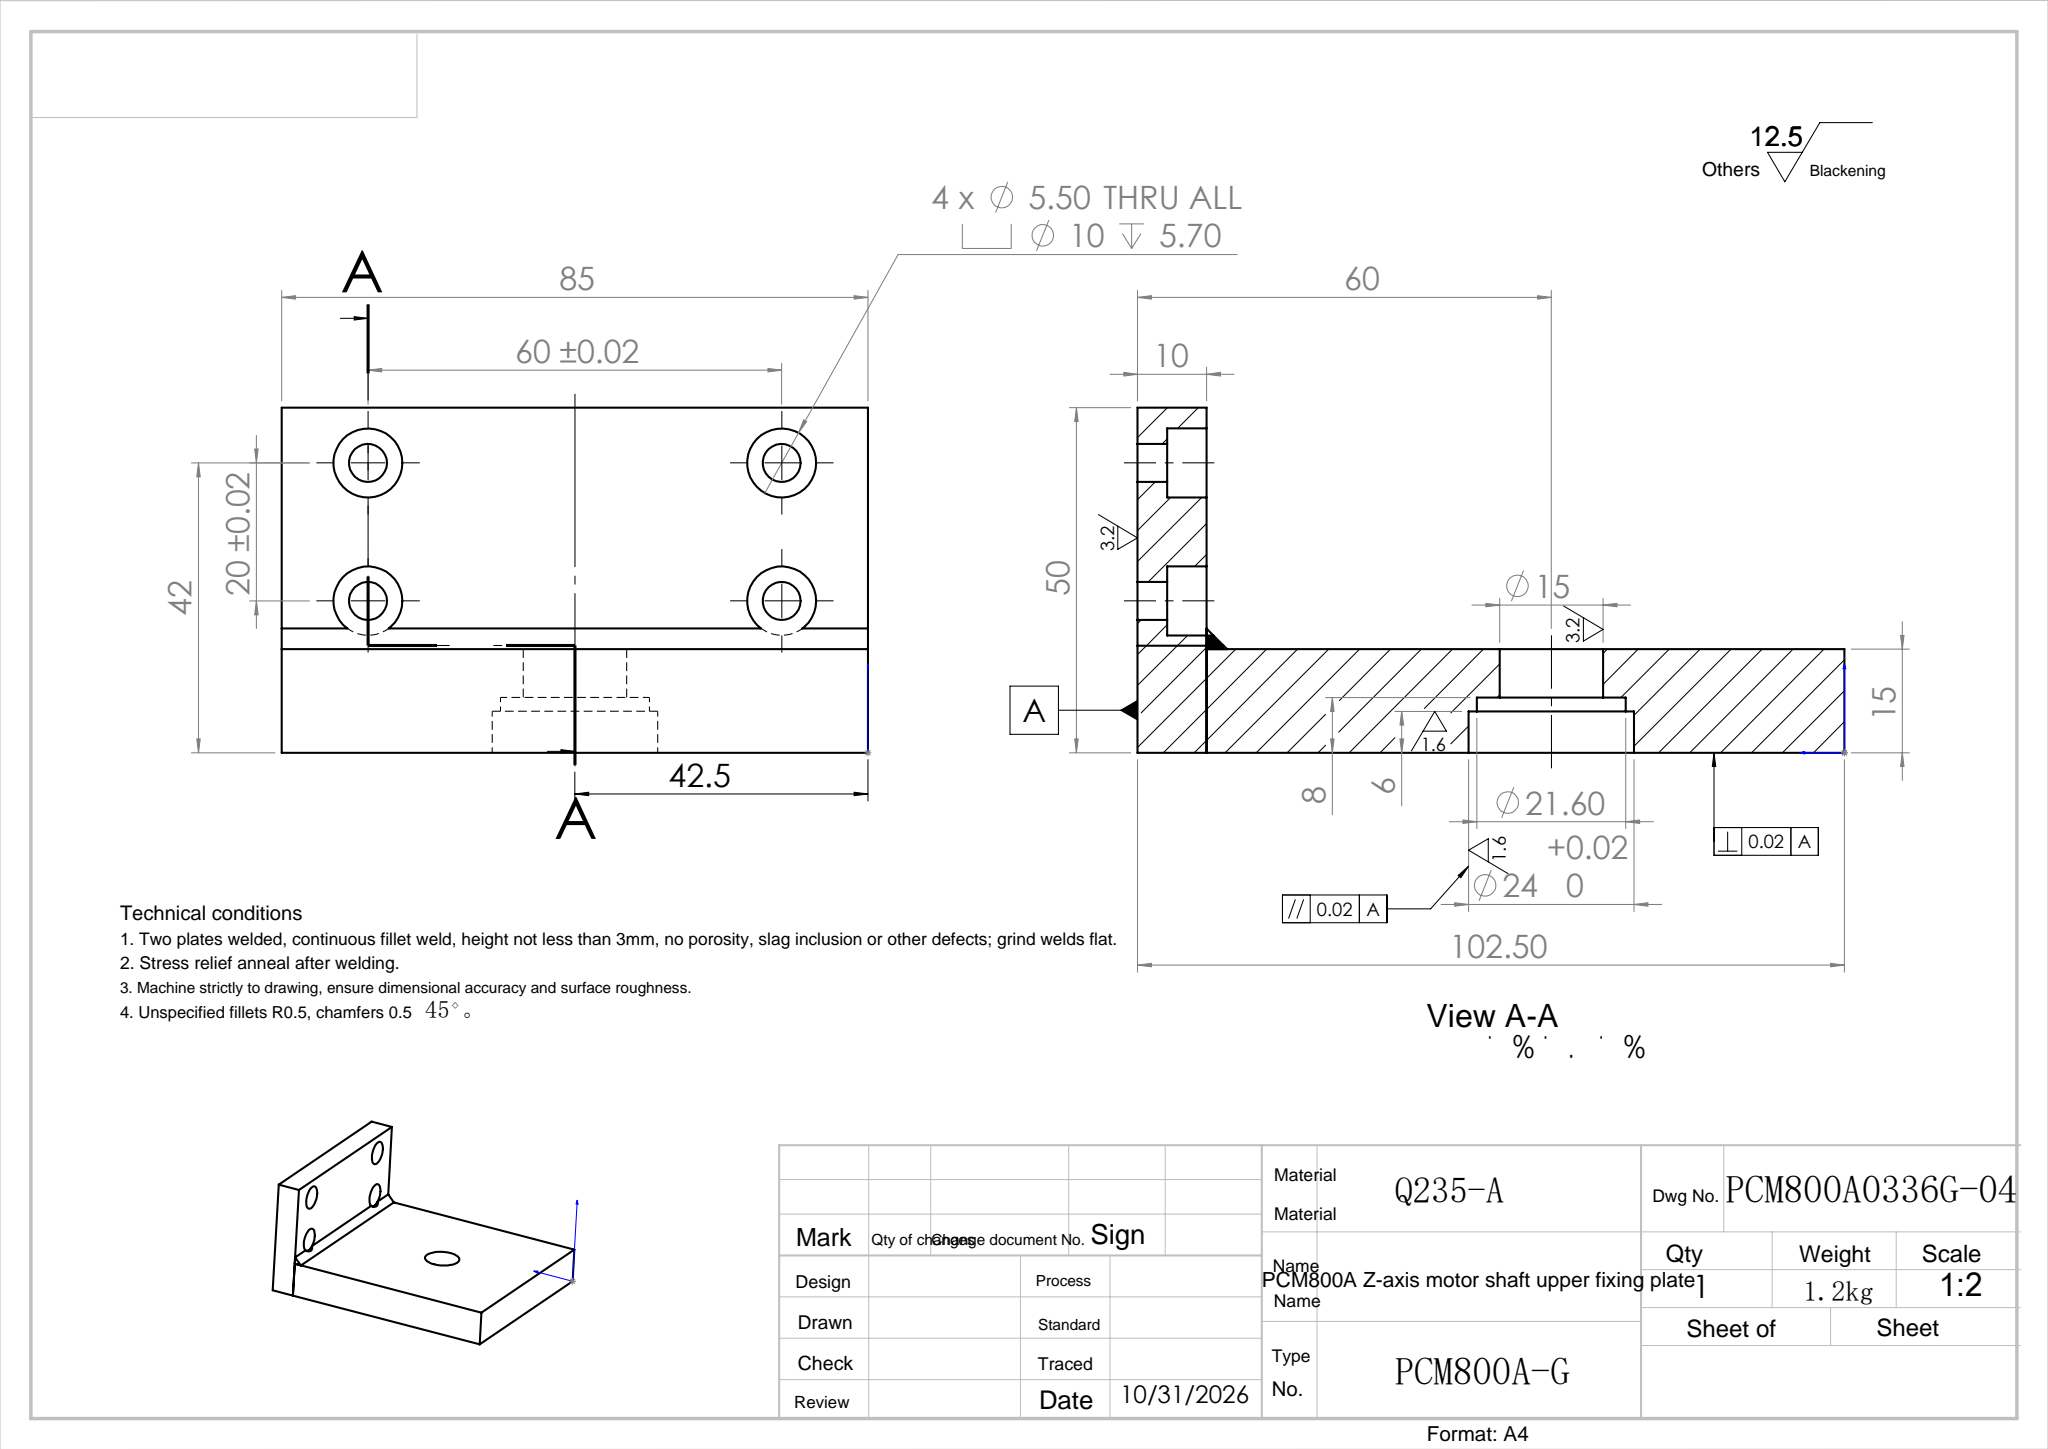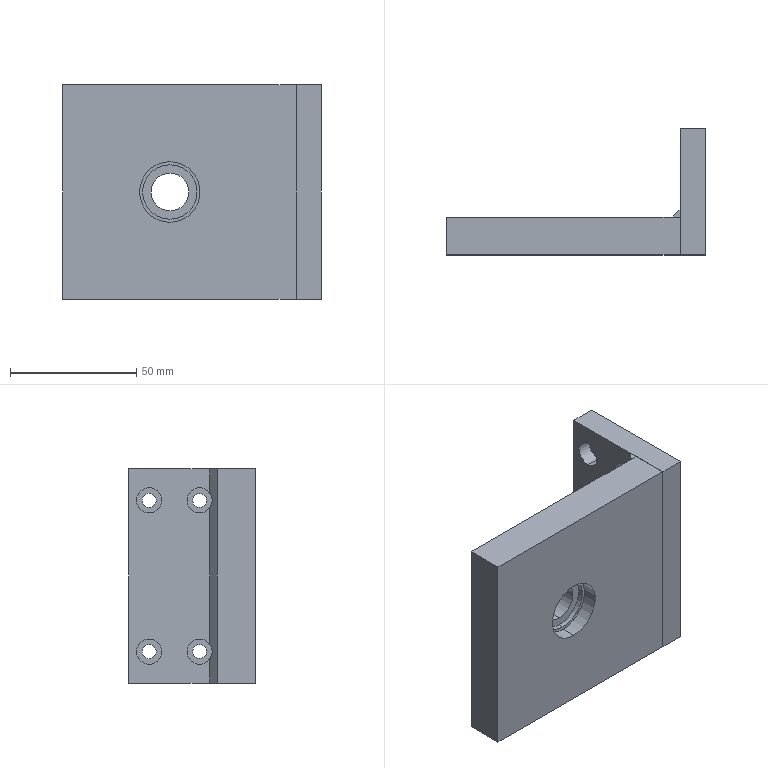Part | SolidWorks | features Cut 3, 3DProfileFeature 1, Boss 1, Extrusion 1, HoleWzd 1, Split 1, WeldBeadFeat 1, WeldmentFeature 1 | 3 solids | 47 faces | box 102.5 x 50 x 85 mm | volume 153933 mm3 | cylinder 24 | plane 23 | commonest cylinder face diameters 10 x10 5.5 x8 15 x2 21.6 x2 24 x2